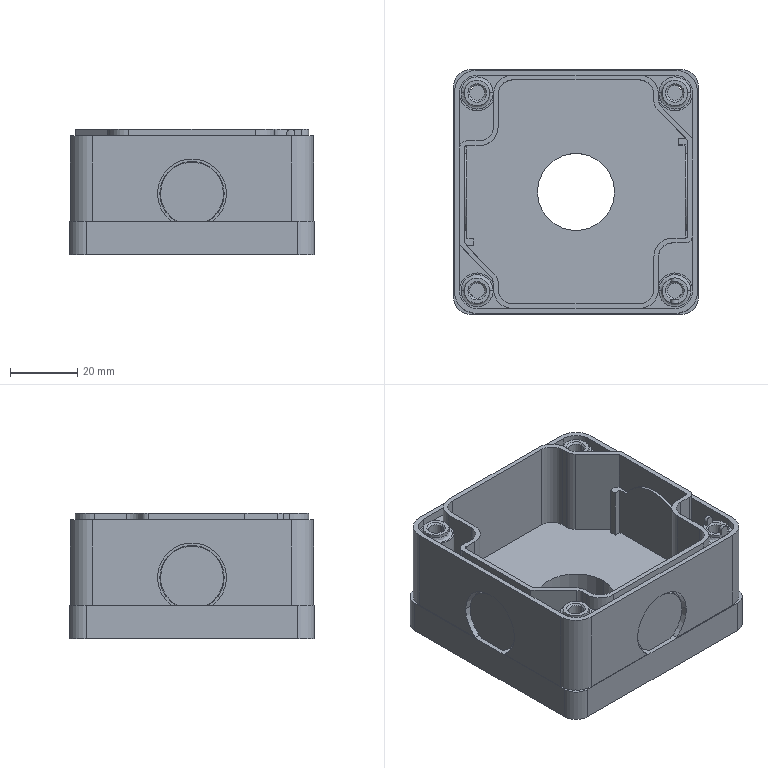Part | STEP file | APT8.024.0682 | 1 solid | 252 faces | box 73 x 73 x 37.5 mm | volume 72648 mm3 | plane 118 | cylinder 101 | cone 17 | spline 16 | commonest cylinder face diameters 7.6 x32 4.6 x10 20.6 x9 4.5 x8 10.6 x8 8.6 x6